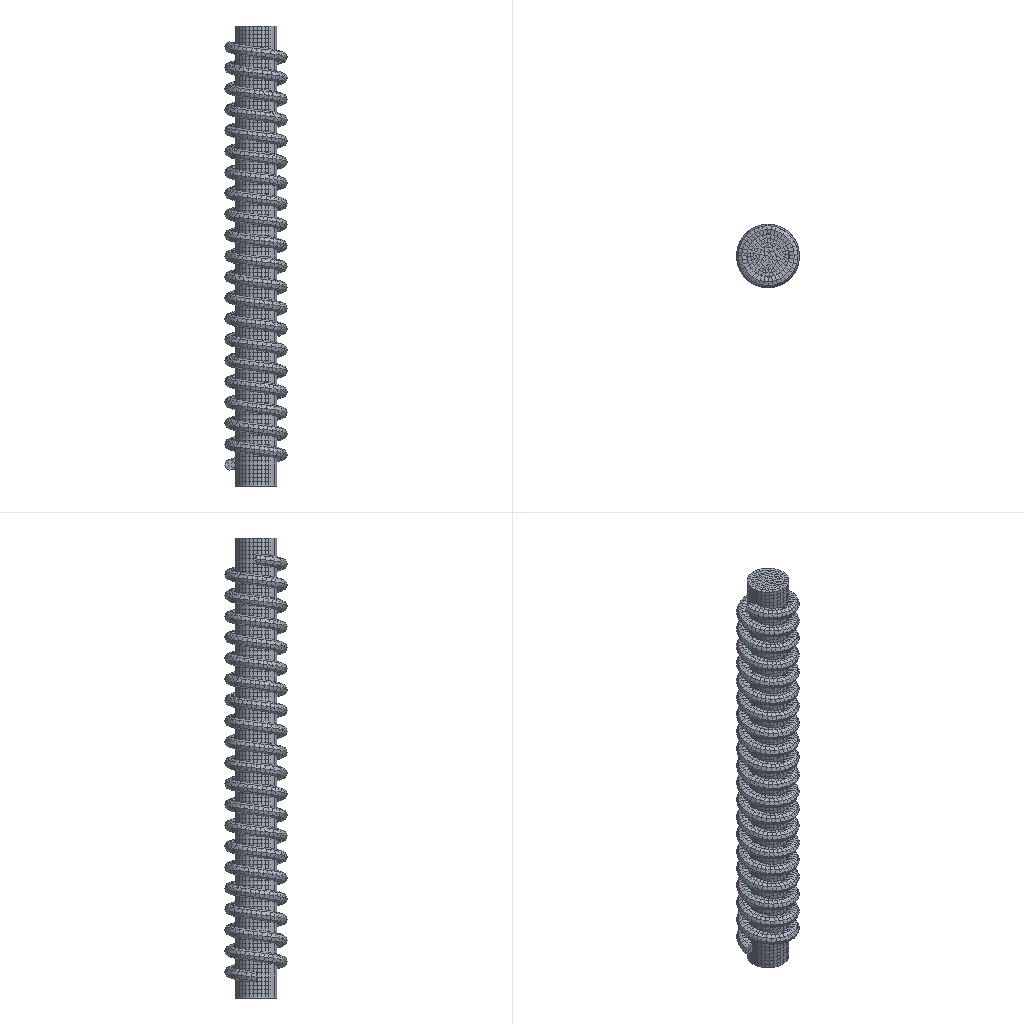Simulation study | abaqus
Set-up summary:
category,name,step,type,value,unit,region
solver,abaqus
solver,version,,,Abaqus/Standard 2020
units,not stated in the deck,,not stated
analysis,deck,,coupled temperature-displacement,coupled temperature-displacement
load_step,Step-1,Step-1,coupled temperature-displacement
load_step,requested,,,1
mesh,nodes,,,22362
mesh,elements,,,16376
element_type,C3D8RT,,solid,16376
load,load commands in deck,,count,3
bc,support commands in deck,,count,1
material,AL,,in results
material,COMPOSITE,,in results
check,setup vs results,,match,"per instance, exact: element labels, types and connectivity; labels of the nodes the elements use; coordinates of those nodes at SINGLE_PRECISION in 1 of 2 instance(s)"
Abaqus input file, long lists of numbers shortened:
*Heading
** Job name: Job-1 Model name: Model-1
** Generated by: Abaqus/CAE 2020
*Preprint, echo=NO, model=NO, history=NO, contact=NO
**
** PARTS
**
*Part, name=bang
*Node
      1,   4.344,  -2.476,           0.
      2,   4.961, -0.6254,           0.
** (15205 more lines like these left out)
*Element, type=C3D8RT
    1,   238,   249,   193,   227,   101,   112,    56,    90
    2,   151,   150,   203,   170,    14,    13,    66,    33
** (13198 more lines like these left out)
*Nset, nset=Set-2, generate
     1,  15207,      1
*Elset, elset=Set-2, generate
     1,  13200,      1
*Nset, nset=Set-11, generate
     1,  15207,      1
*Elset, elset=Set-11, generate
     1,  13200,      1
*Orientation, name=Ori-1
1., 0., 0., 0., 1., 0.
1, 0.
** Section: bang
*Solid Section, elset=Set-11, orientation=Ori-1, material=composite
,
*End Part
**
*Part, name=luoxuanaa
*Node
      1,  -5.366,           0.,   100.884
      2,        -6.25,           0.,       101.25
** (7153 more lines like these left out)
*Element, type=C3D8RT
   1,   17,   16,   18,   10,    8,    7,    9,    1
   2,   13,   12,   18,   14,    4,    3,    9,    5
** (3174 more lines like these left out)
*Nset, nset=Set-2, generate
    1,  7155,     1
*Elset, elset=Set-2, generate
    1,  3176,     1
** Section: al
*Solid Section, elset=Set-2, material=al
,
*End Part
**
**
** ASSEMBLY
**
*Assembly, name=Assembly
**
*Instance, name=bang-1, part=bang
          0.,           0.,          -5.
*End Instance
**
*Instance, name=luoxuanaa-1, part=luoxuanaa
*End Instance
**
*Node
      1,           0., -3.061617e-16,         105.
*Node
      2,           0., 3.061617e-16,          -5.
*Nset, nset=Set-1, instance=bang-1
    12, 15082
*Nset, nset=Set-1, instance=luoxuanaa-1, generate
    1,  7155,     1
*Elset, elset=Set-1, instance=luoxuanaa-1, generate
    1,  3176,     1
*Nset, nset=Set-2, instance=bang-1
    12, 15082
*Nset, nset=Set-2, instance=luoxuanaa-1, generate
    1,  7155,     1
*Elset, elset=Set-2, instance=luoxuanaa-1, generate
    1,  3176,     1
*Nset, nset=Set-3, instance=luoxuanaa-1
    1,    2,    3,    4,    5,    6,    7,    8,    9,   10,   11,   12,   13,   14,   15,   16
   17,   19,   20,   21,   22,   23,   24,   25,   26,   28,   29,   30,   31,   32,   33,   34
** (396 more lines like these left out)
*Elset, elset=Set-3, instance=luoxuanaa-1, generate
    1,  3176,     1
*Nset, nset=Set-6
 1,
*Nset, nset=Set-7
 2,
*Nset, nset=Set-9, instance=bang-1, generate
     1,  15207,      1
*Nset, nset=Set-9, instance=luoxuanaa-1, generate
    1,  7155,     1
*Elset, elset=Set-9, instance=bang-1, generate
     1,  13200,      1
*Elset, elset=Set-9, instance=luoxuanaa-1, generate
    1,  3176,     1
*Nset, nset=m_Set-4
 1,
*Nset, nset=m_Set-5
 2,
*Nset, nset=m_Set-8
 1,
*Elset, elset=_m_Surf-5_S3, internal, instance=bang-1
     2,     3,     5,     6,     7,    11,    12,    16,    18,    23,    25,    26,    27,    28,    29,    31
    33,    34,    38,    40,    42,    50,    65,   112,   122,   123,   125,   126,   127,   131,   132,   136
** (163 more lines like these left out)
*Elset, elset=_m_Surf-5_S5, internal, instance=bang-1
     4,    10,    15,    30,    43,    46,    49,   124,   130,   135,   150,   163,   166,   169,   244,   250
   255,   270,   283,   286,   289,   364,   370,   375,   390,   403,   406,   409,   484,   490,   495,   510
** (47 more lines like these left out)
*Elset, elset=_m_Surf-5_S4, internal, instance=bang-1, generate
    13,  13093,    120
*Surface, type=ELEMENT, name=m_Surf-5
_m_Surf-5_S3, S3
_m_Surf-5_S5, S5
_m_Surf-5_S4, S4
*Elset, elset=_s_Surf-1_S3, internal, instance=luoxuanaa-1, generate
    1,  3176,     1
*Elset, elset=_s_Surf-1_S6, internal, instance=luoxuanaa-1, generate
    1,  3176,     1
*Surface, type=ELEMENT, name=s_Surf-1
_s_Surf-1_S3, S3
_s_Surf-1_S6, S6
*Elset, elset=_s_Surf-6_S1, internal, instance=bang-1, generate
 13081,  13200,      1
*Surface, type=ELEMENT, name=s_Surf-6
_s_Surf-6_S1, S1
*Elset, elset=_s_Surf-7_S2, internal, instance=bang-1, generate
   1,  120,    1
*Surface, type=ELEMENT, name=s_Surf-7
_s_Surf-7_S2, S2
** Constraint: Constraint-1
*Tie, name=Constraint-1, adjust=yes
s_Surf-1, m_Surf-5
** Constraint: Constraint-2
*Coupling, constraint name=Constraint-2, ref node=m_Set-8, surface=s_Surf-6
*Kinematic
** Constraint: Constraint-2-Copy
*Coupling, constraint name=Constraint-2-Copy, ref node=m_Set-5, surface=s_Surf-7
*Kinematic
*End Assembly
*Amplitude, name=Amp-1
             0.,             15.,            900.,            230.,           2700.,             15.
**
** MATERIALS
**
*Material, name=al
*Conductivity
214.,
*Density
 2.7e-09,
*Elastic
72000., 0.28
*Expansion
 2.2e-05,
*Plastic
270.,0.
*Specific Heat
 9e+08,
*Material, name=composite
*Conductivity
40.,
*Density
 2.5e-09,
*Elastic, type=ENGINEERING CONSTANTS
86000.,86000.,86000.,  0.25,  0.35,  0.35, 2000., 2000.
 2000.,
*Expansion
 7e-06,
*Specific Heat
 8e+08,
**
** PREDEFINED FIELDS
**
** Name: Predefined Field-1   Type: Temperature
*Initial Conditions, type=TEMPERATURE
Set-1, 15.
** ----------------------------------------------------------------
**
** STEP: Step-1
**
*Step, name=Step-1, nlgeom=YES, inc=10000
*Coupled Temperature-displacement, creep=none, deltmx=1e+08, stabilize=0.0002, allsdtol=0.05, continue=NO
1., 2700., 0.027, 54.
**
** BOUNDARY CONDITIONS
**
** Name: BC-1 Type: 温度
*Boundary, amplitude=Amp-1
Set-9, 11, 11, 1.
**
** LOADS
**
** Name: Load-1   Type: Concentrated force
*Cload
Set-6, 3, 20.
** Name: Load-1-Copy   Type: Concentrated force
*Cload
Set-7, 3, -20.
**
** OUTPUT REQUESTS
**
*Restart, write, frequency=0
**
** FIELD OUTPUT: F-Output-1
**
*Output, field
*Node Output
CF, NT, RF, RFL, RM, RT, U, V
*Element Output, directions=YES
E, HFL, LE, MISES, MISESMAX, MISESONLY, PE, PEEQ, PEMAG, PRESSONLY, S, SEQUT, SSAVG, TEMP, YIELDPOT
*Contact Output
CDISP, CSTRESS
*Radiation Output
FTEMP,
**
** HISTORY OUTPUT: H-Output-1
**
*Output, history, variable=PRESELECT
*End Step
Results summary:
result,step,,completed,increments=60 time=2700.0/2700.0
result,analysis,,,"coupled temperature-displacement, steady state"
result,last_loadstep,,,1
result,primary field,,,"U, NT11"
result,reaction total,,FX,0.0,model units
result,reaction total,,FY,0.0,model units
result,reaction total,,FZ,0.0,model units